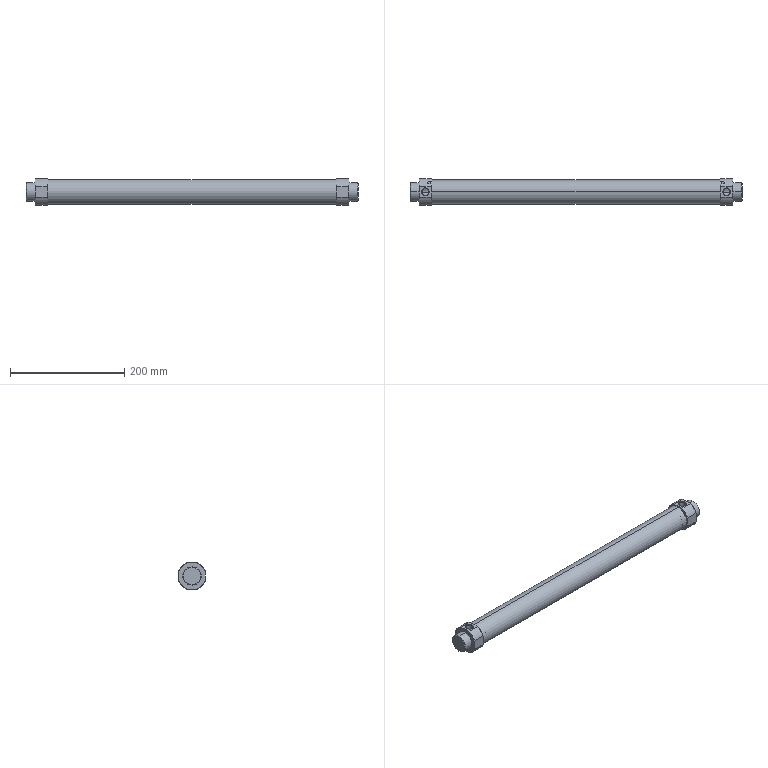Part | STEP file | 11-_RMS40X400(0)-fcv11 | 1 solid | 79 faces | box 582 x 46 x 46 mm | volume 202555 mm3 | cylinder 30 | plane 19 | spline 16 | cone 14 | commonest cylinder face diameters 49.5 x8 5 x4 12 x4 21 x4 32 x4 40 x4